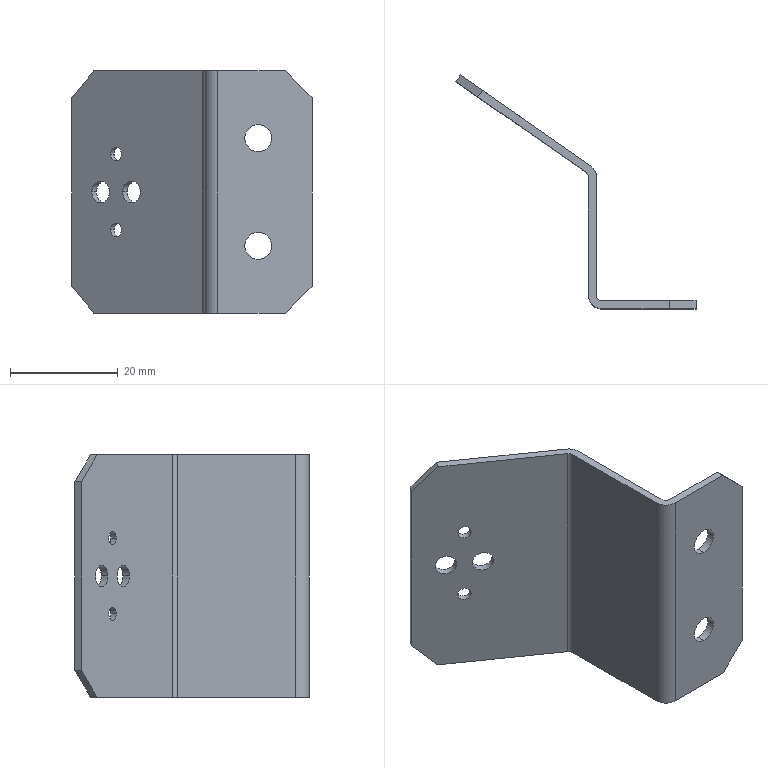Part | STEP file | 1 solid | 34 faces | box 44.575 x 43.436 x 45 mm | volume 4767 mm3 | cylinder 16 | plane 14 | cone 4 | commonest cylinder face diameters 5 x6 2.5 x4 4 x4 2 x2